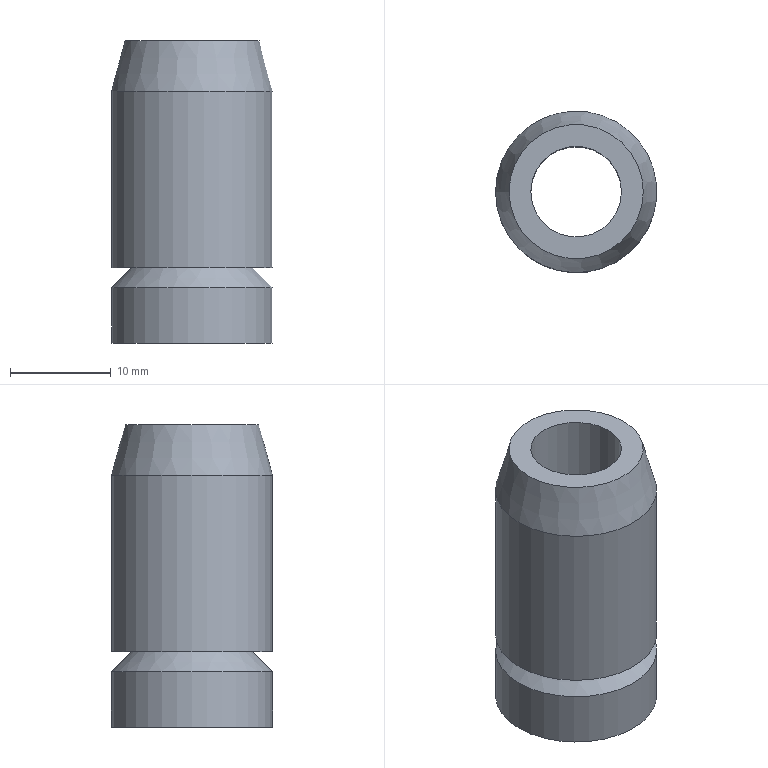Part | NX | features PHBTN70-140-110-Y_3 2 | 1 solid | 8 faces | box 16 x 16 x 30 mm | volume 3872 mm3 | cylinder 3 | plane 3 | cone 2 | commonest cylinder face diameters 16 x2 9 x1
STEP:
#1=CARTESIAN_POINT('',(3590.5,607.5,-113.));
#2=VERTEX_POINT('',#1);
#3=CARTESIAN_POINT('',(3595.,607.5,-113.));
#4=DIRECTION('',(0.,0.,1.));
#5=DIRECTION('',(-1.,0.,0.));
#6=AXIS2_PLACEMENT_3D('',#3,#4,#5);
#7=CIRCLE('',#6,4.5);
#8=EDGE_CURVE('',#2,#2,#7,.T.);
#9=ORIENTED_EDGE('',*,*,#8,.F.);
#10=EDGE_LOOP('',(#9));
#11=FACE_BOUND('',#10,.T.);
#12=CARTESIAN_POINT('',(3590.5,607.5,-83.));
#13=VERTEX_POINT('',#12);
#14=CARTESIAN_POINT('',(3595.,607.5,-83.));
#15=DIRECTION('',(0.,0.,-1.));
#16=DIRECTION('',(-1.,0.,0.));
#17=AXIS2_PLACEMENT_3D('',#14,#15,#16);
#18=CIRCLE('',#17,4.5);
#19=EDGE_CURVE('',#13,#13,#18,.T.);
#20=ORIENTED_EDGE('',*,*,#19,.F.);
#21=EDGE_LOOP('',(#20));
#22=FACE_BOUND('',#21,.T.);
#23=CARTESIAN_POINT('',(3595.,607.5,-98.));
#24=DIRECTION('',(0.,0.,1.));
#25=DIRECTION('',(-1.,0.,0.));
#26=AXIS2_PLACEMENT_3D('',#23,#24,#25);
#27=CYLINDRICAL_SURFACE('',#26,4.5);
#28=ADVANCED_FACE('',(#11,#22),#27,.F.);
#29=CARTESIAN_POINT('',(3587.,607.5,-88.));
#30=VERTEX_POINT('',#29);
#31=CARTESIAN_POINT('',(3595.,607.5,-88.));
#32=DIRECTION('',(0.,0.,1.));
#33=DIRECTION('',(1.,0.,0.));
#34=AXIS2_PLACEMENT_3D('',#31,#32,#33);
#35=CIRCLE('',#34,8.);
#36=EDGE_CURVE('',#30,#30,#35,.T.);
#37=ORIENTED_EDGE('',*,*,#36,.T.);
#38=EDGE_LOOP('',(#37));
#39=FACE_BOUND('',#38,.T.);
#40=CARTESIAN_POINT('',(3588.34,607.5,-83.));
#41=VERTEX_POINT('',#40);
#42=CARTESIAN_POINT('',(3595.,607.5,-83.));
#43=DIRECTION('',(0.,0.,-1.));
#44=DIRECTION('',(1.,0.,0.));
#45=AXIS2_PLACEMENT_3D('',#42,#43,#44);
#46=CIRCLE('',#45,6.66);
#47=EDGE_CURVE('',#41,#41,#46,.T.);
#48=ORIENTED_EDGE('',*,*,#47,.T.);
#49=EDGE_LOOP('',(#48));
#50=FACE_BOUND('',#49,.T.);
#51=CARTESIAN_POINT('',(3595.,607.5,-83.));
#52=DIRECTION('',(0.,0.,-1.));
#53=DIRECTION('',(1.,0.,0.));
#54=AXIS2_PLACEMENT_3D('',#51,#52,#53);
#55=CONICAL_SURFACE('',#54,6.66,0.2618);
#56=ADVANCED_FACE('',(#39,#50),#55,.T.);
#57=CARTESIAN_POINT('',(3587.,607.5,-105.5));
#58=VERTEX_POINT('',#57);
#59=CARTESIAN_POINT('',(3595.,607.5,-105.5));
#60=DIRECTION('',(0.,0.,-1.));
#61=DIRECTION('',(-1.,0.,0.));
#62=AXIS2_PLACEMENT_3D('',#59,#60,#61);
#63=CIRCLE('',#62,8.);
#64=EDGE_CURVE('',#58,#58,#63,.T.);
#65=ORIENTED_EDGE('',*,*,#64,.F.);
#66=EDGE_LOOP('',(#65));
#67=FACE_BOUND('',#66,.T.);
#68=ORIENTED_EDGE('',*,*,#36,.F.);
#69=EDGE_LOOP('',(#68));
#70=FACE_BOUND('',#69,.T.);
#71=CARTESIAN_POINT('',(3595.,607.5,-94.25));
#72=DIRECTION('',(0.,0.,1.));
#73=DIRECTION('',(-1.,0.,0.));
#74=AXIS2_PLACEMENT_3D('',#71,#72,#73);
#75=CYLINDRICAL_SURFACE('',#74,8.);
#76=ADVANCED_FACE('',(#67,#70),#75,.T.);
#77=ORIENTED_EDGE('',*,*,#19,.T.);
#78=EDGE_LOOP('',(#77));
#79=FACE_BOUND('',#78,.T.);
#80=ORIENTED_EDGE('',*,*,#47,.F.);
#81=EDGE_LOOP('',(#80));
#82=FACE_BOUND('',#81,.T.);
#83=CARTESIAN_POINT('',(3595.,607.5,-83.));
#84=DIRECTION('',(0.,0.,1.));
#85=DIRECTION('',(-1.,0.,0.));
#86=AXIS2_PLACEMENT_3D('',#83,#84,#85);
#87=PLANE('',#86);
#88=ADVANCED_FACE('',(#79,#82),#87,.T.);
#89=ORIENTED_EDGE('',*,*,#64,.T.);
#90=EDGE_LOOP('',(#89));
#91=FACE_BOUND('',#90,.T.);
#92=CARTESIAN_POINT('',(3589.,607.5,-105.5));
#93=VERTEX_POINT('',#92);
#94=CARTESIAN_POINT('',(3595.,607.5,-105.5));
#95=DIRECTION('',(0.,0.,-1.));
#96=DIRECTION('',(1.,0.,0.));
#97=AXIS2_PLACEMENT_3D('',#94,#95,#96);
#98=CIRCLE('',#97,6.);
#99=EDGE_CURVE('',#93,#93,#98,.T.);
#100=ORIENTED_EDGE('',*,*,#99,.F.);
#101=EDGE_LOOP('',(#100));
#102=FACE_BOUND('',#101,.T.);
#103=CARTESIAN_POINT('',(3595.,607.5,-105.5));
#104=DIRECTION('',(0.,0.,-1.));
#105=DIRECTION('',(1.,0.,0.));
#106=AXIS2_PLACEMENT_3D('',#103,#104,#105);
#107=PLANE('',#106);
#108=ADVANCED_FACE('',(#91,#102),#107,.T.);
#109=CARTESIAN_POINT('',(3587.,607.5,-107.5));
#110=VERTEX_POINT('',#109);
#111=CARTESIAN_POINT('',(3595.,607.5,-107.5));
#112=DIRECTION('',(0.,0.,1.));
#113=DIRECTION('',(1.,0.,0.));
#114=AXIS2_PLACEMENT_3D('',#111,#112,#113);
#115=CIRCLE('',#114,8.);
#116=EDGE_CURVE('',#110,#110,#115,.T.);
#117=ORIENTED_EDGE('',*,*,#116,.T.);
#118=EDGE_LOOP('',(#117));
#119=FACE_BOUND('',#118,.T.);
#120=ORIENTED_EDGE('',*,*,#99,.T.);
#121=EDGE_LOOP('',(#120));
#122=FACE_BOUND('',#121,.T.);
#123=CARTESIAN_POINT('',(3595.,607.5,-105.5));
#124=DIRECTION('',(0.,0.,-1.));
#125=DIRECTION('',(1.,0.,0.));
#126=AXIS2_PLACEMENT_3D('',#123,#124,#125);
#127=CONICAL_SURFACE('',#126,6.,0.7854);
#128=ADVANCED_FACE('',(#119,#122),#127,.T.);
#129=CARTESIAN_POINT('',(3587.,607.5,-113.));
#130=VERTEX_POINT('',#129);
#131=CARTESIAN_POINT('',(3595.,607.5,-113.));
#132=DIRECTION('',(0.,0.,-1.));
#133=DIRECTION('',(-1.,0.,0.));
#134=AXIS2_PLACEMENT_3D('',#131,#132,#133);
#135=CIRCLE('',#134,8.);
#136=EDGE_CURVE('',#130,#130,#135,.T.);
#137=ORIENTED_EDGE('',*,*,#136,.F.);
#138=EDGE_LOOP('',(#137));
#139=FACE_BOUND('',#138,.T.);
#140=ORIENTED_EDGE('',*,*,#116,.F.);
#141=EDGE_LOOP('',(#140));
#142=FACE_BOUND('',#141,.T.);
#143=CARTESIAN_POINT('',(3595.,607.5,-109.25));
#144=DIRECTION('',(0.,0.,1.));
#145=DIRECTION('',(-1.,0.,0.));
#146=AXIS2_PLACEMENT_3D('',#143,#144,#145);
#147=CYLINDRICAL_SURFACE('',#146,8.);
#148=ADVANCED_FACE('',(#139,#142),#147,.T.);
#149=ORIENTED_EDGE('',*,*,#8,.T.);
#150=EDGE_LOOP('',(#149));
#151=FACE_BOUND('',#150,.T.);
#152=ORIENTED_EDGE('',*,*,#136,.T.);
#153=EDGE_LOOP('',(#152));
#154=FACE_BOUND('',#153,.T.);
#155=CARTESIAN_POINT('',(3595.,607.5,-113.));
#156=DIRECTION('',(0.,0.,-1.));
#157=DIRECTION('',(1.,0.,0.));
#158=AXIS2_PLACEMENT_3D('',#155,#156,#157);
#159=PLANE('',#158);
#160=ADVANCED_FACE('',(#151,#154),#159,.T.);
#161=CLOSED_SHELL('',(#28,#56,#76,#88,#108,#128,#148,#160));
#162=MANIFOLD_SOLID_BREP('',#161);
#163=(LENGTH_UNIT()NAMED_UNIT(*)SI_UNIT(.MILLI.,.METRE.));
#164=UNCERTAINTY_MEASURE_WITH_UNIT(LENGTH_MEASURE(0.00001),#163,'','');
#165=(NAMED_UNIT(*)PLANE_ANGLE_UNIT()SI_UNIT($,.RADIAN.));
#166=(NAMED_UNIT(*)SI_UNIT($,.STERADIAN.)SOLID_ANGLE_UNIT());
#167=(GEOMETRIC_REPRESENTATION_CONTEXT(3)GLOBAL_UNCERTAINTY_ASSIGNED_CONTEXT((#164))GLOBAL_UNIT_ASSIGNED_CONTEXT((#163,#165,#166))REPRESENTATION_CONTEXT('',''));
#168=ADVANCED_BREP_SHAPE_REPRESENTATION('',(#162),#167);